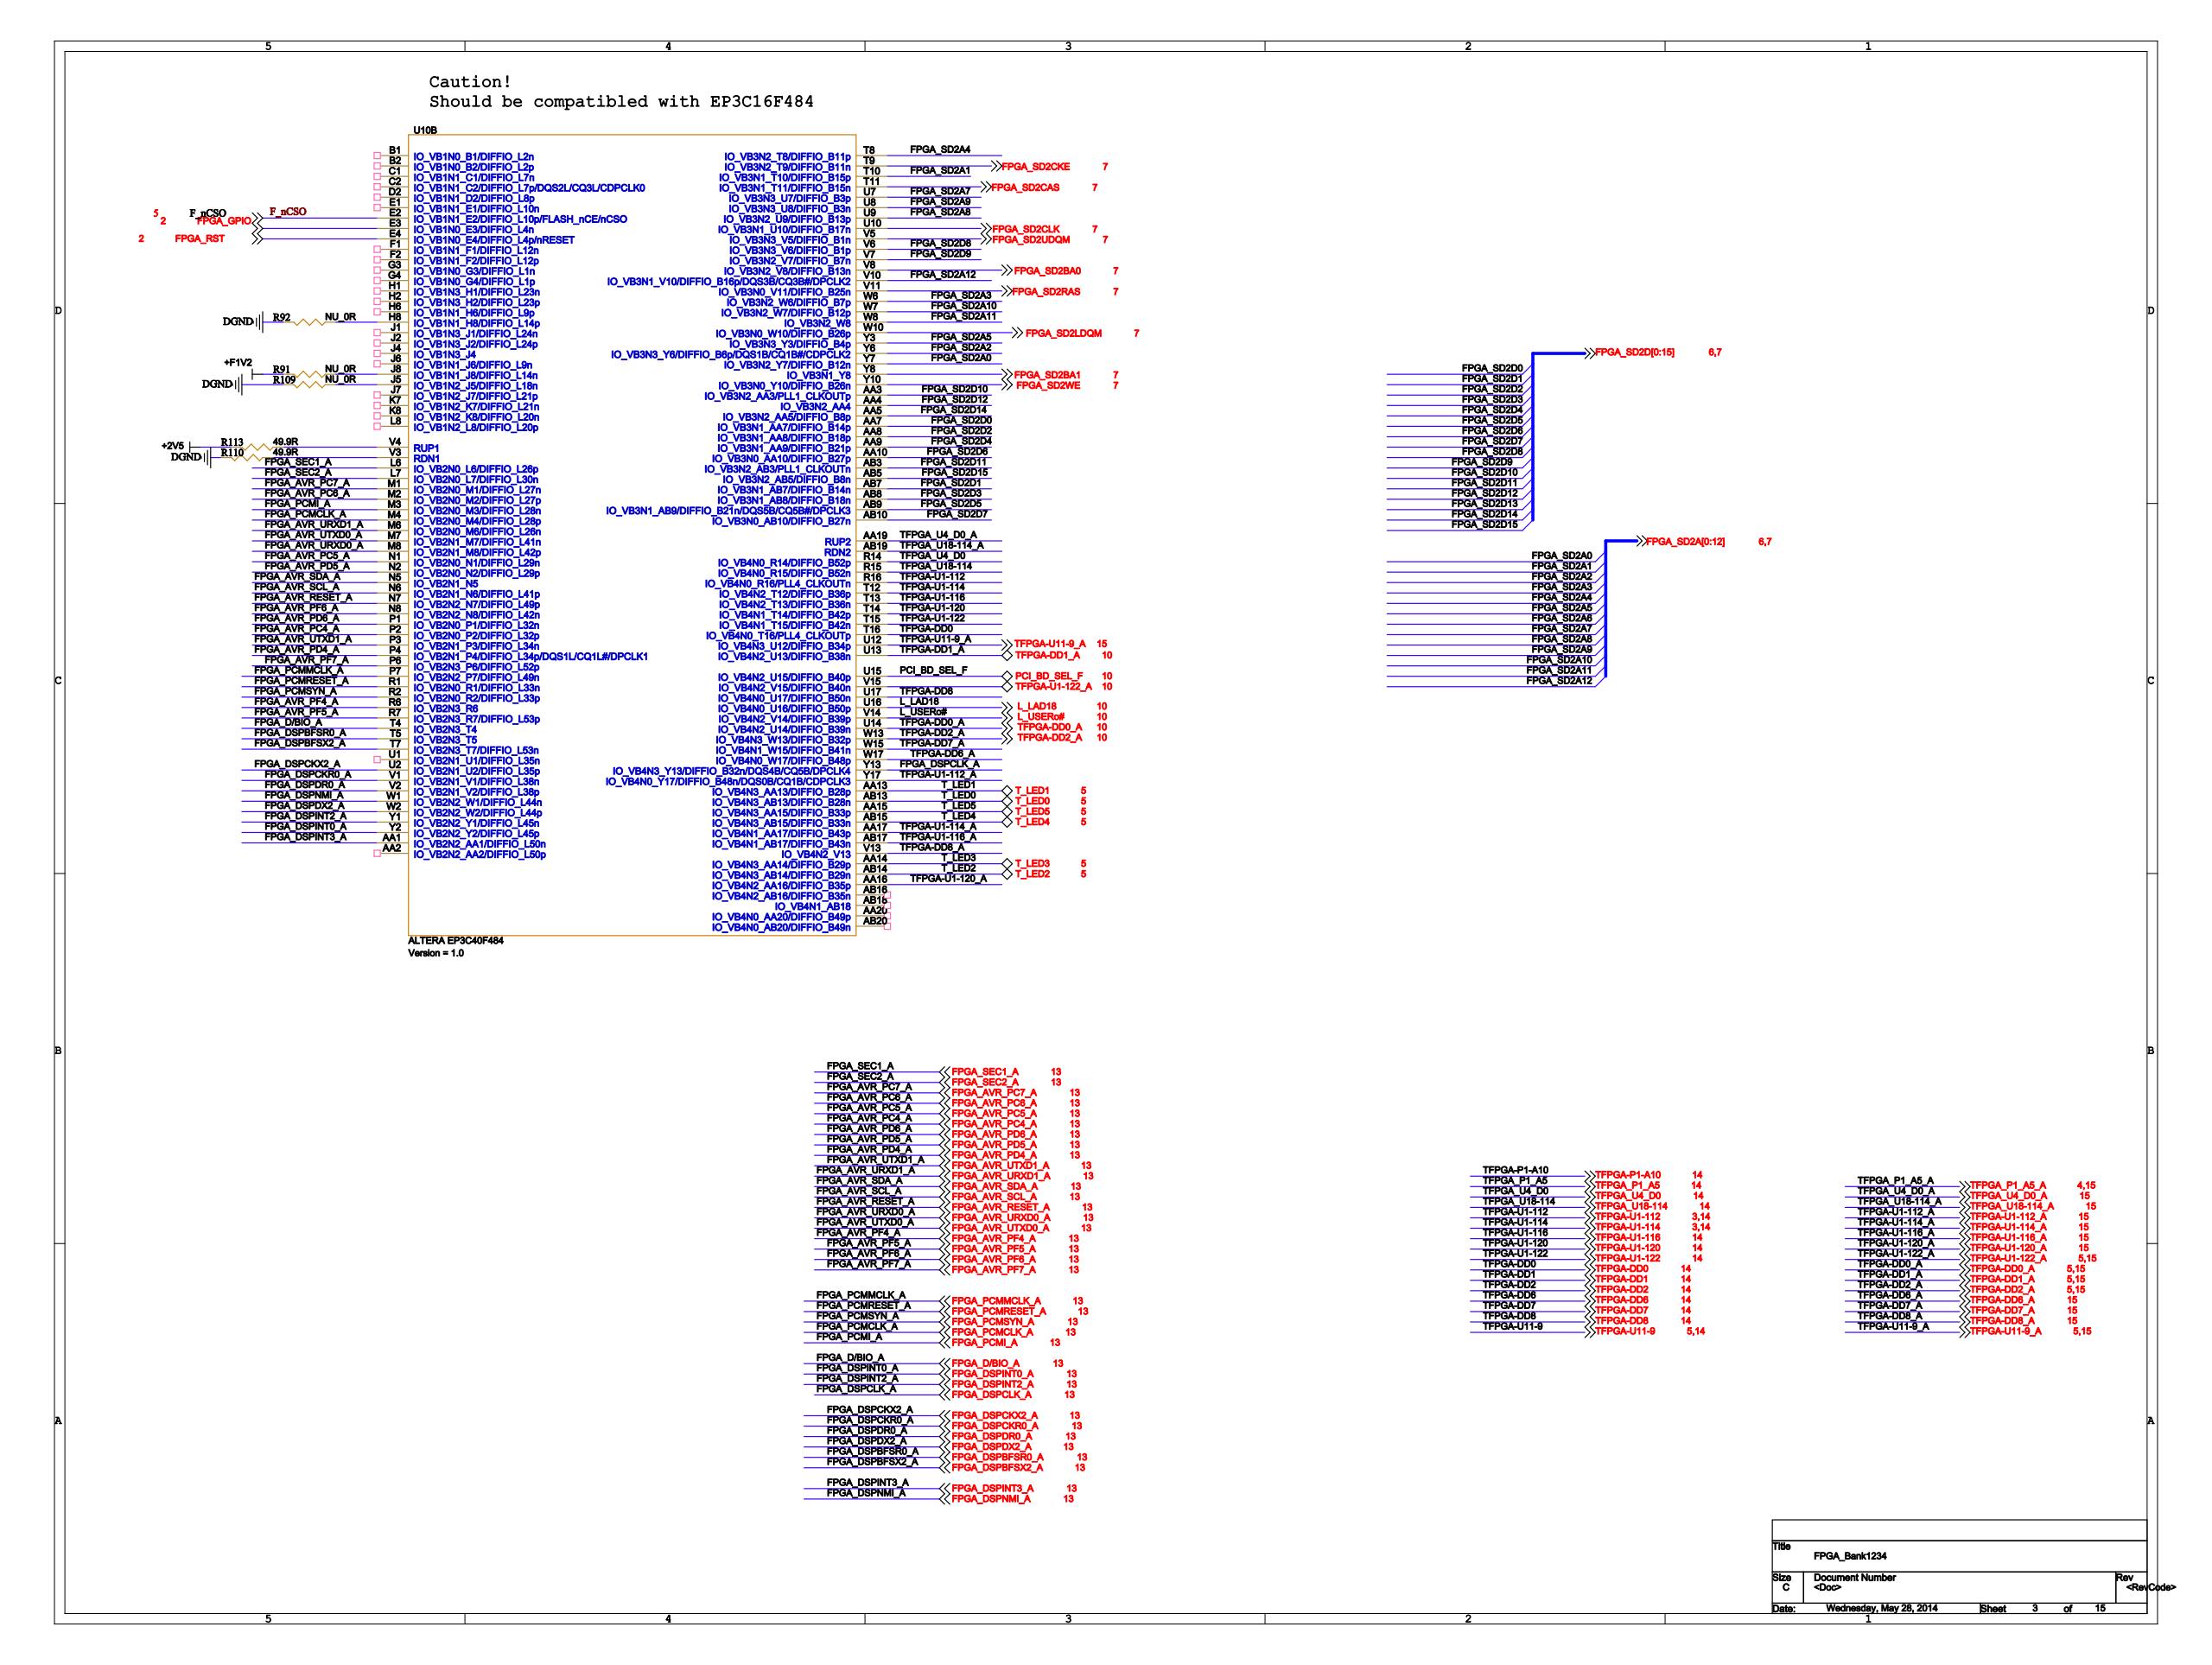Circuit board | Cadence Allegro | 669 parts | 806 nets | one sheet of the schematic
Parts on this sheet (reference | value | footprint):
J2 | CompactPCI-J1 | CPCI_J1_4
J6 | CPCI_AB110_J5 | CPCI_J2_5
R91 | NU_0R | R0603
R92 | NU_0R | R0603
R109 | NU_0R | R0603
R110 | 49.9R | R0603
R113 | 49.9R | R0603
U10 | EP3C40F484C8N | FBGA484
Nets of these parts (net: part-pin ...):
DGND: R92-2 R109-2 R110-2 J2-F1 J2-F2 J6-F1 J6-F2
FPGA_SEC2_A: U10-L7
FPGA_SEC1_A: U10-L6
+F1V2: R91-2
FPGA_GPIO: U10-E3
FPGA_RST: U10-E4
N2355442: R92-1 U10-H8
N61307220: R91-1 U10-J8
N61307221: R109-1 U10-J5
FPGA_AVR_PC7_A: U10-M1
FPGA_AVR_PC6_A: U10-M2
FPGA_PCMI_A: U10-M3
FPGA_PCMCLK_A: U10-M4
FPGA_AVR_URXD1_A: U10-M6
FPGA_AVR_PC5_A: U10-N1
FPGA_AVR_PD5_A: U10-N2
FPGA_AVR_PD6_A: U10-P1
FPGA_AVR_PC4_A: U10-P2
FPGA_PCMRESET_A: U10-R1
FPGA_PCMSYN_A: U10-R2
FPGA_AVR_UTXD0_A: U10-M7
FPGA_AVR_URXD0_A: U10-M8
FPGA_AVR_SDA_A: U10-N5
FPGA_AVR_SCL_A: U10-N6
FPGA_AVR_UTXD1_A: U10-P3
FPGA_AVR_PD4_A: U10-P4
FPGA_DSPCKX2_A: U10-U2
FPGA_DSPCKR0_A: U10-V1
FPGA_DSPDR0_A: U10-V2
FPGA_DSPINT3_A: U10-AA1
FPGA_AVR_RESET_A: U10-N7
FPGA_AVR_PF6_A: U10-N8
FPGA_PCMMCLK_A: U10-P7
FPGA_DSPNMI_A: U10-W1
FPGA_DSPDX2_A: U10-W2
FPGA_DSPINT2_A: U10-Y1
FPGA_DSPINT0_A: U10-Y2
FPGA_AVR_PF7_A: U10-P6
FPGA_AVR_PF4_A: U10-R6
FPGA_AVR_PF5_A: U10-R7
FPGA_D/BIO_A: U10-T4
FPGA_DSPBFSR0_A: U10-T5
FPGA_DSPBFSX2_A: U10-T7
FPGA_SD2D6: U10-AA10
FPGA_SD2D7: U10-AB10
FPGA_SD2RAS: U10-V11
FPGA_SD2LDQM: U10-W10
FPGA_SD2WE: U10-Y10
FPGA_SD2D0: U10-AA7
FPGA_SD2D2: U10-AA8
FPGA_SD2D4: U10-AA9
FPGA_SD2D1: U10-AB7
FPGA_SD2D3: U10-AB8
FPGA_SD2D5: U10-AB9
FPGA_SD2A1: U10-T10
FPGA_SD2CAS: U10-T11
FPGA_SD2CLK: U10-U10
FPGA_SD2A12: U10-V10
FPGA_SD2BA1: U10-Y8
FPGA_SD2D10: U10-AA3
FPGA_SD2D12: U10-AA4
FPGA_SD2D14: U10-AA5
FPGA_SD2D11: U10-AB3
FPGA_SD2D15: U10-AB5
FPGA_SD2A4: U10-T8
FPGA_SD2CKE: U10-T9
FPGA_SD2A8: U10-U9
FPGA_SD2D9: U10-V7
FPGA_SD2BA0: U10-V8
FPGA_SD2A3: U10-W6
FPGA_SD2A10: U10-W7
FPGA_SD2A11: U10-W8
FPGA_SD2A0: U10-Y7
FPGA_SD2A7: U10-U7
FPGA_SD2A9: U10-U8
FPGA_SD2UDQM: U10-V5
FPGA_SD2D8: U10-V6
FPGA_SD2A5: U10-Y3
FPGA_SD2A2: U10-Y6
TFPGA_U4_D0: U10-R14
TFPGA_U18-114: U10-R15
TFPGA-U1-112: U10-R16
TFPGA-DD0: U10-T16
L_LAD18: U10-U16
TFPGA-DD8: U10-U17
TFPGA-DD6_A: U10-W17
TFPGA-U1-112_A: U10-Y17
TFPGA-U1-114_A: U10-AA17
TFPGA-U1-116_A: U10-AB17
TFPGA-U1-120: U10-T14
TFPGA-U1-122: U10-T15
TFPGA-DD7_A: U10-W15
TFPGA-U1-120_A: U10-AA16
TFPGA-U1-114: U10-T12
TFPGA-U1-116: U10-T13
TFPGA-DD1_A: U10-U13
TFPGA-DD0_A: U10-U14
PCI_BD_SEL_F: U10-U15
TFPGA-DD8_A: U10-V13
TFPGA-U1-122_A: U10-V15
T_LED1: U10-AA13
T_LED3: U10-AA14
T_LED5: U10-AA15
T_LED0: U10-AB13
T_LED2: U10-AB14
T_LED4: U10-AB15
TFPGA-U11-9_A: U10-U12
TFPGA-DD2_A: U10-W13
FPGA_DSPCLK_A: U10-Y13
N56587028: R110-1 U10-V3
TFPGA_U18-114_A: U10-AB19
N56589481: R113-1 U10-V4
TFPGA_U4_D0_A: U10-AA19
+2V5: R113-2